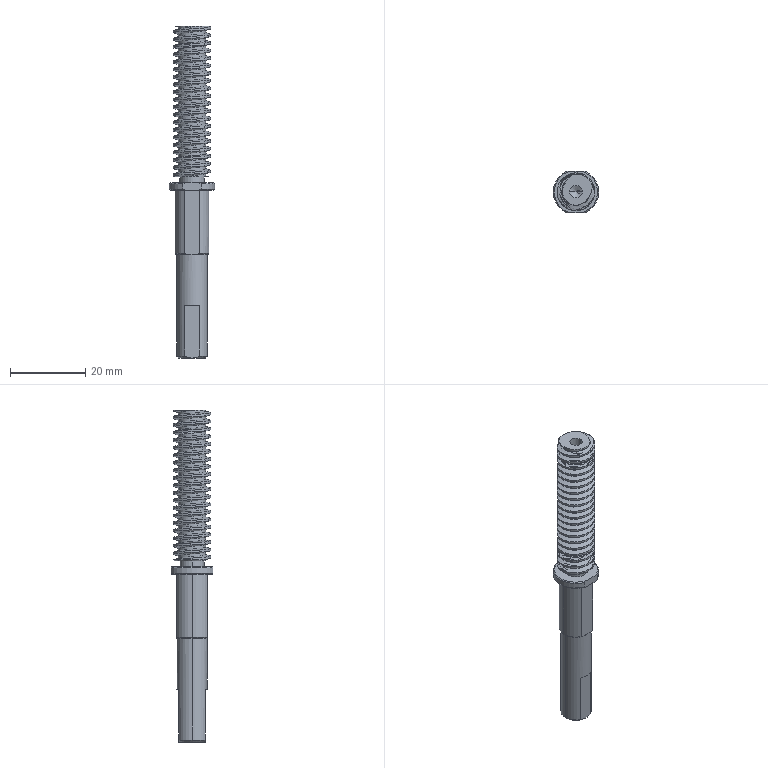Part | NX | features BREP 1 | 1 solid | 92 faces | box 12 x 11 x 88 mm | volume 4646 mm3 | cylinder 56 | cone 18 | plane 16 | spline 2 | commonest cylinder face diameters 10 x41 9 x3 12 x3 3.3 x2 4.2 x2 6.5 x2